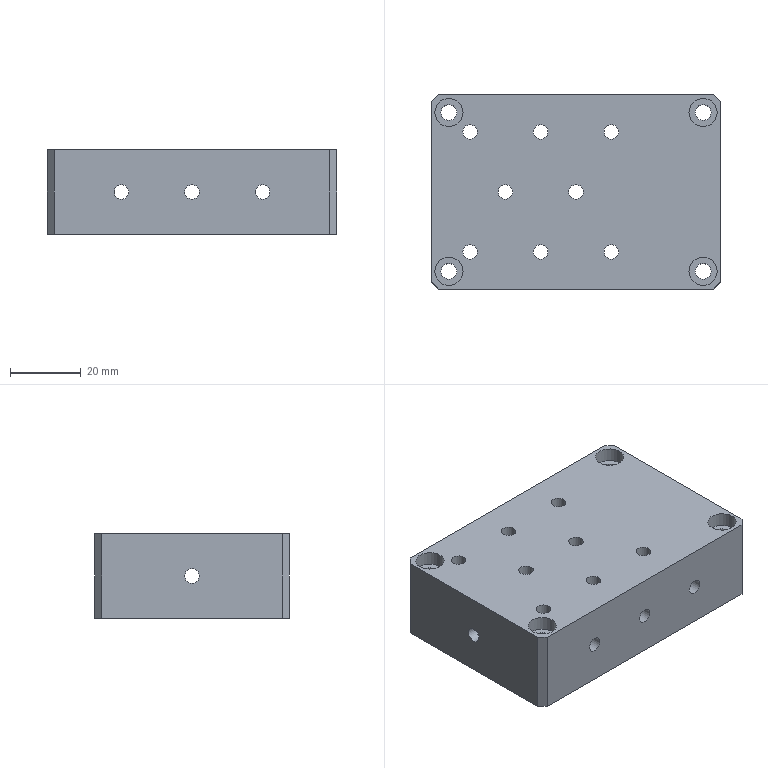NC program | NX | posted with a generic post | part box 82 x 55 x 24 mm
Lines 1802 to 2085 of 2085:
(ZLEVEL_PROFILE_COPY_1 , TOOL : D10JING)
N3578 T14 M6
N3580 G54
N3582 G17 G0 G90 X35.332 Y-32.5 B0. C0. S9500 M3
N3584 G43 Z30. H14
N3586 Z1.5
N3588 G94 G1 X-39.549 Z-2.424 F1000.
N3590 X-40.925 Y-32.147 Z-2.499
N3592 X-42.148 Y-31.423 Z-2.573
N3594 X-44.923 Y-28.648 Z-2.779
N3596 X-45.647 Y-27.425 Z-2.853
N3598 X-46. Y-26.049 Z-2.928
N3600 Y26.049 Z-5.658
N3602 X-45.647 Y27.425 Z-5.733
N3604 X-44.923 Y28.648 Z-5.807
N3606 X-42.148 Y31.423 Z-6.013
N3608 X-40.925 Y32.147 Z-6.087
N3610 X-39.549 Y32.5 Z-6.162
N3612 X39.549 Z-10.307
N3614 X40.925 Y32.147 Z-10.382
N3616 X42.148 Y31.423 Z-10.456
N3618 X44.923 Y28.648 Z-10.662
N3620 X45.647 Y27.425 Z-10.736
N3622 X46. Y26.049 Z-10.811
N3624 Y-26.049 Z-13.541
N3626 X45.647 Y-27.425 Z-13.615
N3628 X44.923 Y-28.648 Z-13.69
N3630 X42.148 Y-31.423 Z-13.896
N3632 X40.925 Y-32.147 Z-13.97
N3634 X39.549 Y-32.5 Z-14.045
N3636 X-39.549 Z-18.19
N3638 X-40.925 Y-32.147 Z-18.264
N3640 X-42.148 Y-31.423 Z-18.339
N3642 X-44.923 Y-28.648 Z-18.545
N3644 X-45.647 Y-27.425 Z-18.619
N3646 X-46. Y-26.049 Z-18.693
N3648 Y26.049 Z-21.424
N3650 X-45.647 Y27.425 Z-21.498
N3652 X-44.923 Y28.648 Z-21.573
N3654 X-42.148 Y31.423 Z-21.778
N3656 X-40.925 Y32.147 Z-21.853
N3658 X-39.549 Y32.5 Z-21.927
N3660 X0. Z-24.
N3662 X39. F1200.
N3664 G2 X42.536 Y31.036 R5.
N3666 G1 X44.536 Y29.036
N3668 G2 X46. Y25.5 R5.
N3670 G1 Y-25.5
N3672 G2 X44.536 Y-29.036 R5.
N3674 G1 X42.536 Y-31.036
N3676 G2 X39. Y-32.5 R5.
N3678 G1 X-39.
N3680 G2 X-42.536 Y-31.036 R5.
N3682 G1 X-44.536 Y-29.036
N3684 G2 X-46. Y-25.5 R5.
N3686 G1 Y25.5
N3688 G2 X-44.536 Y29.036 R5.
N3690 G1 X-42.536 Y31.036
N3692 G2 X-39. Y32.5 R5.
N3694 G1 X0.
N3696 Z-22.5
N3698 G0 Z30.
N3700 M5
(HOLE_MILLING , TOOL : D6)
N3702 T12 M6
N3704 G54
N3706 G17 G0 G90 X-36. Y22.5 B0. C0. S9500 M3
N3708 G43 Z30. H12
N3710 Z0.5
N3712 G94 G3 X-35.5 Y22. R0.5 F1500.
N3714 X-35. Y22.5 R0.5
N3716 X-35. Y22.5 Z0. I-1. J0.
N3718 X-35. Y22.5 Z-0.5 I-1. J0.
N3720 X-35. Y22.5 Z-1. I-1. J0.
N3722 X-35. Y22.5 Z-1.5 I-1. J0.
N3724 X-35. Y22.5 Z-2. I-1. J0.
N3726 X-35. Y22.5 Z-2.5 I-1. J0.
N3728 X-35. Y22.5 Z-3. I-1. J0.
N3730 X-35. Y22.5 Z-3.5 I-1. J0.
N3732 X-35. Y22.5 Z-4. I-1. J0.
N3734 X-36. Y23.5 R1.
N3736 X-35. Y22.5 R-1.
N3738 X-35.5 Y23. R0.5
N3740 X-36. Y22.5 R0.5
N3742 G0 Z30.
N3744 Y-22.5
N3746 Z0.5
N3748 G3 X-35.5 Y-23. R0.5
N3750 X-35. Y-22.5 R0.5
N3752 X-35. Y-22.5 Z0. I-1. J0.
N3754 X-35. Y-22.5 Z-0.5 I-1. J0.
N3756 X-35. Y-22.5 Z-1. I-1. J0.
N3758 X-35. Y-22.5 Z-1.5 I-1. J0.
N3760 X-35. Y-22.5 Z-2. I-1. J0.
N3762 X-35. Y-22.5 Z-2.5 I-1. J0.
N3764 X-35. Y-22.5 Z-3. I-1. J0.
N3766 X-35. Y-22.5 Z-3.5 I-1. J0.
N3768 X-35. Y-22.5 Z-4. I-1. J0.
N3770 X-36. Y-21.5 R1.
N3772 X-35. Y-22.5 R-1.
N3774 X-35.5 Y-22. R0.5
N3776 X-36. Y-22.5 R0.5
N3778 G0 Z30.
N3780 X36.
N3782 Z0.5
N3784 G3 X36.5 Y-23. R0.5
N3786 X37. Y-22.5 R0.5
N3788 X37. Y-22.5 Z0. I-1. J0.
N3790 X37. Y-22.5 Z-0.5 I-1. J0.
N3792 X37. Y-22.5 Z-1. I-1. J0.
N3794 X37. Y-22.5 Z-1.5 I-1. J0.
N3796 X37. Y-22.5 Z-2. I-1. J0.
N3798 X37. Y-22.5 Z-2.5 I-1. J0.
N3800 X37. Y-22.5 Z-3. I-1. J0.
N3802 X37. Y-22.5 Z-3.5 I-1. J0.
N3804 X37. Y-22.5 Z-4. I-1. J0.
N3806 X36. Y-21.5 R1.
N3808 X37. Y-22.5 R-1.
N3810 X36.5 Y-22. R0.5
N3812 X36. Y-22.5 R0.5
N3814 G0 Z30.
N3816 Y22.5
N3818 Z0.5
N3820 G3 X36.5 Y22. R0.5
N3822 X37. Y22.5 R0.5
N3824 X37. Y22.5 Z0. I-1. J0.
N3826 X37. Y22.5 Z-0.5 I-1. J0.
N3828 X37. Y22.5 Z-1. I-1. J0.
N3830 X37. Y22.5 Z-1.5 I-1. J0.
N3832 X37. Y22.5 Z-2. I-1. J0.
N3834 X37. Y22.5 Z-2.5 I-1. J0.
N3836 X37. Y22.5 Z-3. I-1. J0.
N3838 X37. Y22.5 Z-3.5 I-1. J0.
N3840 X37. Y22.5 Z-4. I-1. J0.
N3842 X36. Y23.5 R1.
N3844 X37. Y22.5 R-1.
N3846 X36.5 Y23. R0.5
N3848 X36. Y22.5 R0.5
N3850 G0 Z30.
N3852 M5
(PLANAR_MILL_COPY_COPY_COPY , TOOL : D6A45)
N3854 T01 M6
N3856 G54
N3858 G17 G0 G90 X36.866 Y25.1 B0. C0. S9500 M3
N3860 G43 Z30. H1
N3862 Z0.5
N3864 G94 G1 Z-1. F1250.
N3866 G3 X36. Y25.6 R1.
N3868 X32.9 Y22.5 R3.1
N3870 X36. Y25.6 R-3.1
N3872 X35.134 Y25.1 R1.
N3874 G1 Z0.5
N3876 G0 Z30.
N3878 X10.866 Y17.667
N3880 Z0.5
N3882 G1 Z-1.
N3884 G3 X10. Y18.167 R1.
N3886 X8.833 Y17. R1.167
N3888 X10. Y18.167 R-1.167
N3890 X9.134 Y17.667 R1.
N3892 G1 Z0.5
N3894 G0 Z30.
N3896 X-9.134
N3898 Z0.5
N3900 G1 Z-1.
N3902 G3 X-10. Y18.167 R1.
N3904 X-11.167 Y17. R1.167
N3906 X-10. Y18.167 R-1.167
N3908 X-10.866 Y17.667 R1.
N3910 G1 Z0.5
N3912 G0 Z30.
N3914 X-35.134 Y25.1
N3916 Z0.5
N3918 G1 Z-1.
N3920 G3 X-36. Y25.6 R1.
N3922 X-39.1 Y22.5 R3.1
N3924 X-36. Y25.6 R-3.1
N3926 X-36.866 Y25.1 R1.
N3928 G1 Z0.5
N3930 G0 Z30.
N3932 X-29.134 Y17.667
N3934 Z0.5
N3936 G1 Z-1.
N3938 G3 X-30. Y18.167 R1.
N3940 X-31.167 Y17. R1.167
N3942 X-30. Y18.167 R-1.167
N3944 X-30.866 Y17.667 R1.
N3946 G1 Z0.5
N3948 G0 Z30.
N3950 X-20.667 Y0.866
N3952 Z0.5
N3954 G1 Z-1.
N3956 G3 X-21.167 Y0. R1.
N3958 X-20. Y-1.167 R1.167
N3960 X-21.167 Y0. R-1.167
N3962 X-20.667 Y-0.866 R1.
N3964 G1 Z0.5
N3966 G0 Z30.
N3968 X-30.866 Y-17.667
N3970 Z0.5
N3972 G1 Z-1.
N3974 G3 X-30. Y-18.167 R1.
N3976 X-28.833 Y-17. R1.167
N3978 X-30. Y-18.167 R-1.167
N3980 X-29.134 Y-17.667 R1.
N3982 G1 Z0.5
N3984 G0 Z30.
N3986 X-38.6 Y-21.634
N3988 Z0.5
N3990 G1 Z-1.
N3992 G3 X-39.1 Y-22.5 R1.
N3994 X-36. Y-25.6 R3.1
N3996 X-39.1 Y-22.5 R-3.1
N3998 X-38.6 Y-23.366 R1.
N4000 G1 Z0.5
N4002 G0 Z30.
N4004 X-10.866 Y-17.667
N4006 Z0.5
N4008 G1 Z-1.
N4010 G3 X-10. Y-18.167 R1.
N4012 X-8.833 Y-17. R1.167
N4014 X-10. Y-18.167 R-1.167
N4016 X-9.134 Y-17.667 R1.
N4018 G1 Z0.5
N4020 G0 Z30.
N4022 X0.866 Y-28.9
N4024 Z0.5
N4026 G1 Z-1.
N4028 G3 X0. Y-28.4 R1.
N4030 G1 X-39.
N4032 G2 X-39.636 Y-28.136 R0.9
N4034 G1 X-41.636 Y-26.136
N4036 G2 X-41.9 Y-25.5 R0.9
N4038 G1 Y25.5
N4040 G2 X-41.636 Y26.136 R0.9
N4042 G1 X-39.636 Y28.136
N4044 G2 X-39. Y28.4 R0.9
N4046 G1 X39.
N4048 G2 X39.636 Y28.136 R0.9
N4050 G1 X41.636 Y26.136
N4052 G2 X41.9 Y25.5 R0.9
N4054 G1 Y-25.5
N4056 G2 X41.636 Y-26.136 R0.9
N4058 G1 X39.636 Y-28.136
N4060 G2 X39. Y-28.4 R0.9
N4062 G1 X0.
N4064 G3 X-0.866 Y-28.9 R1.
N4066 G1 Z0.5
N4068 G0 Z30.
N4070 Y-0.667
N4072 Z0.5
N4074 G1 Z-1.
N4076 G3 X0. Y-1.167 R1.
N4078 X1.167 Y0. R1.167
N4080 X0. Y-1.167 R-1.167
N4082 X0.866 Y-0.667 R1.
N4084 G1 Z0.5
N4086 G0 Z30.
N4088 X9.134 Y-17.667
N4090 Z0.5
N4092 G1 Z-1.
N4094 G3 X10. Y-18.167 R1.
N4096 X11.167 Y-17. R1.167
N4098 X10. Y-18.167 R-1.167
N4100 X10.866 Y-17.667 R1.
N4102 G1 Z0.5
N4104 G0 Z30.
N4106 X35.134 Y-25.1
N4108 Z0.5
N4110 G1 Z-1.
N4112 G3 X36. Y-25.6 R1.
N4114 X39.1 Y-22.5 R3.1
N4116 X36. Y-25.6 R-3.1
N4118 X36.866 Y-25.1 R1.
N4120 G1 Z0.5
N4122 G0 Z30.
N4124 M5
N4126 M2